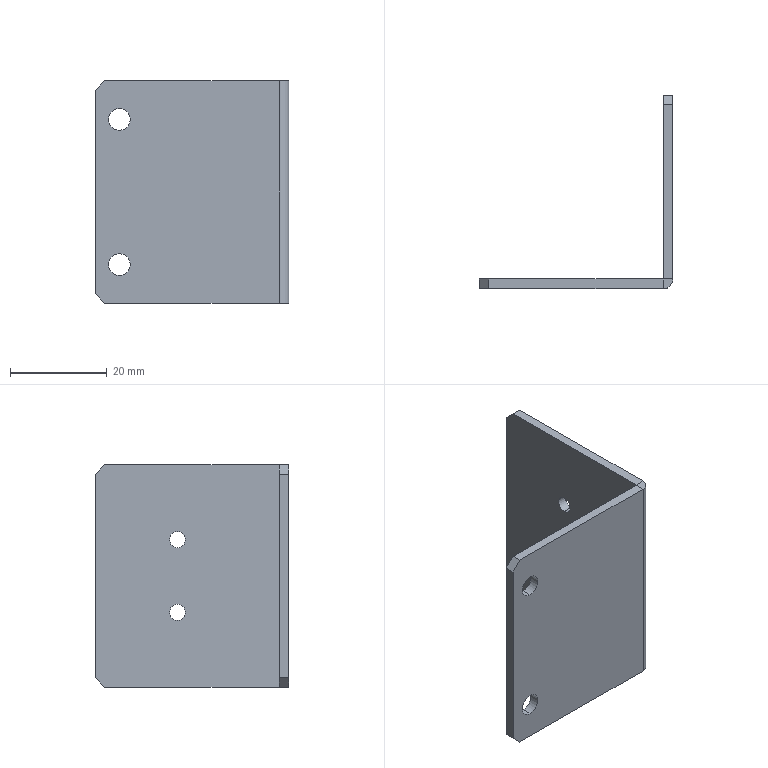Part | NX | features BREP 1 | 1 solid | 26 faces | box 40 x 40 x 46 mm | volume 7022 mm3 | plane 16 | cylinder 10 | commonest cylinder face diameters 3.3 x4 4.5 x4 0.02 x1 4.02 x1
STEP:
#1=CARTESIAN_POINT('',(0.,23.,5.85));
#2=VERTEX_POINT('',#1);
#3=CARTESIAN_POINT('',(0.,23.,9.15));
#4=VERTEX_POINT('',#3);
#5=CARTESIAN_POINT('',(0.,23.,7.5));
#6=DIRECTION('',(-1.,0.,0.));
#7=DIRECTION('',(0.,0.,1.));
#8=AXIS2_PLACEMENT_3D('',#5,#6,#7);
#9=CIRCLE('',#8,1.65);
#10=EDGE_CURVE('',#2,#4,#9,.T.);
#11=ORIENTED_EDGE('',*,*,#10,.F.);
#12=CARTESIAN_POINT('',(-2.,23.,5.85));
#13=VERTEX_POINT('',#12);
#14=CARTESIAN_POINT('',(-2.,23.,5.85));
#15=DIRECTION('',(-1.,0.,0.));
#16=VECTOR('',#15,1000.);
#17=LINE('',#14,#16);
#18=EDGE_CURVE('',#13,#2,#17,.F.);
#19=ORIENTED_EDGE('',*,*,#18,.F.);
#20=CARTESIAN_POINT('',(-2.,23.,9.15));
#21=VERTEX_POINT('',#20);
#22=CARTESIAN_POINT('',(-2.,23.,7.5));
#23=DIRECTION('',(-1.,0.,0.));
#24=DIRECTION('',(0.,0.,1.));
#25=AXIS2_PLACEMENT_3D('',#22,#23,#24);
#26=CIRCLE('',#25,1.65);
#27=EDGE_CURVE('',#13,#21,#26,.T.);
#28=ORIENTED_EDGE('',*,*,#27,.T.);
#29=CARTESIAN_POINT('',(-2.,23.,9.15));
#30=DIRECTION('',(-1.,0.,0.));
#31=VECTOR('',#30,1000.);
#32=LINE('',#29,#31);
#33=EDGE_CURVE('',#21,#4,#32,.F.);
#34=ORIENTED_EDGE('',*,*,#33,.T.);
#35=EDGE_LOOP('',(#11,#19,#28,#34));
#36=FACE_BOUND('',#35,.T.);
#37=CARTESIAN_POINT('',(-2.,23.,7.5));
#38=DIRECTION('',(-1.,0.,0.));
#39=DIRECTION('',(0.,0.,1.));
#40=AXIS2_PLACEMENT_3D('',#37,#38,#39);
#41=CYLINDRICAL_SURFACE('',#40,1.65);
#42=ADVANCED_FACE('',(#36),#41,.F.);
#43=CARTESIAN_POINT('',(0.,23.,-9.15));
#44=VERTEX_POINT('',#43);
#45=CARTESIAN_POINT('',(0.,23.,-5.85));
#46=VERTEX_POINT('',#45);
#47=CARTESIAN_POINT('',(0.,23.,-7.5));
#48=DIRECTION('',(-1.,0.,0.));
#49=DIRECTION('',(0.,0.,1.));
#50=AXIS2_PLACEMENT_3D('',#47,#48,#49);
#51=CIRCLE('',#50,1.65);
#52=EDGE_CURVE('',#44,#46,#51,.T.);
#53=ORIENTED_EDGE('',*,*,#52,.F.);
#54=CARTESIAN_POINT('',(-2.,23.,-9.15));
#55=VERTEX_POINT('',#54);
#56=CARTESIAN_POINT('',(-2.,23.,-9.15));
#57=DIRECTION('',(-1.,0.,0.));
#58=VECTOR('',#57,1000.);
#59=LINE('',#56,#58);
#60=EDGE_CURVE('',#55,#44,#59,.F.);
#61=ORIENTED_EDGE('',*,*,#60,.F.);
#62=CARTESIAN_POINT('',(-2.,23.,-5.85));
#63=VERTEX_POINT('',#62);
#64=CARTESIAN_POINT('',(-2.,23.,-7.5));
#65=DIRECTION('',(-1.,0.,0.));
#66=DIRECTION('',(0.,0.,1.));
#67=AXIS2_PLACEMENT_3D('',#64,#65,#66);
#68=CIRCLE('',#67,1.65);
#69=EDGE_CURVE('',#55,#63,#68,.T.);
#70=ORIENTED_EDGE('',*,*,#69,.T.);
#71=CARTESIAN_POINT('',(-2.,23.,-5.85));
#72=DIRECTION('',(-1.,0.,0.));
#73=VECTOR('',#72,1000.);
#74=LINE('',#71,#73);
#75=EDGE_CURVE('',#63,#46,#74,.F.);
#76=ORIENTED_EDGE('',*,*,#75,.T.);
#77=EDGE_LOOP('',(#53,#61,#70,#76));
#78=FACE_BOUND('',#77,.T.);
#79=CARTESIAN_POINT('',(-2.,23.,-7.5));
#80=DIRECTION('',(-1.,0.,0.));
#81=DIRECTION('',(0.,0.,1.));
#82=AXIS2_PLACEMENT_3D('',#79,#80,#81);
#83=CYLINDRICAL_SURFACE('',#82,1.65);
#84=ADVANCED_FACE('',(#78),#83,.F.);
#85=CARTESIAN_POINT('',(-35.,0.,-12.75));
#86=VERTEX_POINT('',#85);
#87=CARTESIAN_POINT('',(-35.,0.,-17.25));
#88=VERTEX_POINT('',#87);
#89=CARTESIAN_POINT('',(-35.,0.,-15.));
#90=DIRECTION('',(0.,-1.,0.));
#91=DIRECTION('',(1.,0.,0.));
#92=AXIS2_PLACEMENT_3D('',#89,#90,#91);
#93=CIRCLE('',#92,2.25);
#94=EDGE_CURVE('',#86,#88,#93,.T.);
#95=ORIENTED_EDGE('',*,*,#94,.T.);
#96=CARTESIAN_POINT('',(-35.,2.,-17.25));
#97=VERTEX_POINT('',#96);
#98=CARTESIAN_POINT('',(-35.,2.,-17.25));
#99=DIRECTION('',(0.,1.,0.));
#100=VECTOR('',#99,1000.);
#101=LINE('',#98,#100);
#102=EDGE_CURVE('',#97,#88,#101,.F.);
#103=ORIENTED_EDGE('',*,*,#102,.F.);
#104=CARTESIAN_POINT('',(-35.,2.,-12.75));
#105=VERTEX_POINT('',#104);
#106=CARTESIAN_POINT('',(-35.,2.,-15.));
#107=DIRECTION('',(0.,1.,0.));
#108=DIRECTION('',(0.,0.,1.));
#109=AXIS2_PLACEMENT_3D('',#106,#107,#108);
#110=CIRCLE('',#109,2.25);
#111=EDGE_CURVE('',#97,#105,#110,.T.);
#112=ORIENTED_EDGE('',*,*,#111,.T.);
#113=CARTESIAN_POINT('',(-35.,2.,-12.75));
#114=DIRECTION('',(0.,1.,0.));
#115=VECTOR('',#114,1000.);
#116=LINE('',#113,#115);
#117=EDGE_CURVE('',#105,#86,#116,.F.);
#118=ORIENTED_EDGE('',*,*,#117,.T.);
#119=EDGE_LOOP('',(#95,#103,#112,#118));
#120=FACE_BOUND('',#119,.T.);
#121=CARTESIAN_POINT('',(-35.,2.,-15.));
#122=DIRECTION('',(0.,1.,0.));
#123=DIRECTION('',(0.,0.,1.));
#124=AXIS2_PLACEMENT_3D('',#121,#122,#123);
#125=CYLINDRICAL_SURFACE('',#124,2.25);
#126=ADVANCED_FACE('',(#120),#125,.F.);
#127=CARTESIAN_POINT('',(-35.,0.,17.25));
#128=VERTEX_POINT('',#127);
#129=CARTESIAN_POINT('',(-35.,0.,12.75));
#130=VERTEX_POINT('',#129);
#131=CARTESIAN_POINT('',(-35.,0.,15.));
#132=DIRECTION('',(0.,-1.,0.));
#133=DIRECTION('',(1.,0.,0.));
#134=AXIS2_PLACEMENT_3D('',#131,#132,#133);
#135=CIRCLE('',#134,2.25);
#136=EDGE_CURVE('',#128,#130,#135,.T.);
#137=ORIENTED_EDGE('',*,*,#136,.T.);
#138=CARTESIAN_POINT('',(-35.,2.,12.75));
#139=VERTEX_POINT('',#138);
#140=CARTESIAN_POINT('',(-35.,2.,12.75));
#141=DIRECTION('',(0.,1.,0.));
#142=VECTOR('',#141,1000.);
#143=LINE('',#140,#142);
#144=EDGE_CURVE('',#139,#130,#143,.F.);
#145=ORIENTED_EDGE('',*,*,#144,.F.);
#146=CARTESIAN_POINT('',(-35.,2.,17.25));
#147=VERTEX_POINT('',#146);
#148=CARTESIAN_POINT('',(-35.,2.,15.));
#149=DIRECTION('',(0.,1.,0.));
#150=DIRECTION('',(0.,0.,1.));
#151=AXIS2_PLACEMENT_3D('',#148,#149,#150);
#152=CIRCLE('',#151,2.25);
#153=EDGE_CURVE('',#139,#147,#152,.T.);
#154=ORIENTED_EDGE('',*,*,#153,.T.);
#155=CARTESIAN_POINT('',(-35.,2.,17.25));
#156=DIRECTION('',(0.,1.,0.));
#157=VECTOR('',#156,1000.);
#158=LINE('',#155,#157);
#159=EDGE_CURVE('',#147,#128,#158,.F.);
#160=ORIENTED_EDGE('',*,*,#159,.T.);
#161=EDGE_LOOP('',(#137,#145,#154,#160));
#162=FACE_BOUND('',#161,.T.);
#163=CARTESIAN_POINT('',(-35.,2.,15.));
#164=DIRECTION('',(0.,1.,0.));
#165=DIRECTION('',(0.,0.,1.));
#166=AXIS2_PLACEMENT_3D('',#163,#164,#165);
#167=CYLINDRICAL_SURFACE('',#166,2.25);
#168=ADVANCED_FACE('',(#162),#167,.F.);
#169=CARTESIAN_POINT('',(-2.01,0.,23.));
#170=VERTEX_POINT('',#169);
#171=CARTESIAN_POINT('',(-2.01,2.,23.));
#172=VERTEX_POINT('',#171);
#173=CARTESIAN_POINT('',(-2.01,0.,23.));
#174=DIRECTION('',(0.,1.,0.));
#175=VECTOR('',#174,1000.);
#176=LINE('',#173,#175);
#177=EDGE_CURVE('',#170,#172,#176,.T.);
#178=ORIENTED_EDGE('',*,*,#177,.F.);
#179=CARTESIAN_POINT('',(0.,2.01,23.));
#180=VERTEX_POINT('',#179);
#181=CARTESIAN_POINT('',(-2.01,2.01,23.));
#182=DIRECTION('',(0.,0.,-1.));
#183=DIRECTION('',(1.,0.,0.));
#184=AXIS2_PLACEMENT_3D('',#181,#182,#183);
#185=CIRCLE('',#184,2.01);
#186=EDGE_CURVE('',#180,#170,#185,.T.);
#187=ORIENTED_EDGE('',*,*,#186,.F.);
#188=CARTESIAN_POINT('',(-2.,2.01,23.));
#189=VERTEX_POINT('',#188);
#190=CARTESIAN_POINT('',(-2.,2.01,23.));
#191=DIRECTION('',(1.,0.,0.));
#192=VECTOR('',#191,1000.);
#193=LINE('',#190,#192);
#194=EDGE_CURVE('',#189,#180,#193,.T.);
#195=ORIENTED_EDGE('',*,*,#194,.F.);
#196=CARTESIAN_POINT('',(-2.01,2.01,23.));
#197=DIRECTION('',(0.,0.,-1.));
#198=DIRECTION('',(1.,0.,0.));
#199=AXIS2_PLACEMENT_3D('',#196,#197,#198);
#200=CIRCLE('',#199,0.01);
#201=EDGE_CURVE('',#189,#172,#200,.T.);
#202=ORIENTED_EDGE('',*,*,#201,.T.);
#203=EDGE_LOOP('',(#178,#187,#195,#202));
#204=FACE_BOUND('',#203,.T.);
#205=CARTESIAN_POINT('',(-2.01,0.,23.));
#206=DIRECTION('',(0.,0.,1.));
#207=DIRECTION('',(1.,0.,0.));
#208=AXIS2_PLACEMENT_3D('',#205,#206,#207);
#209=PLANE('',#208);
#210=ADVANCED_FACE('',(#204),#209,.T.);
#211=CARTESIAN_POINT('',(-38.,2.,23.));
#212=VERTEX_POINT('',#211);
#213=CARTESIAN_POINT('',(0.,2.,23.));
#214=DIRECTION('',(-1.,0.,0.));
#215=VECTOR('',#214,1000.);
#216=LINE('',#213,#215);
#217=EDGE_CURVE('',#172,#212,#216,.T.);
#218=ORIENTED_EDGE('',*,*,#217,.T.);
#219=CARTESIAN_POINT('',(-38.,0.,23.));
#220=VERTEX_POINT('',#219);
#221=CARTESIAN_POINT('',(-38.,2.01,23.));
#222=DIRECTION('',(0.,-1.,0.));
#223=VECTOR('',#222,1000.);
#224=LINE('',#221,#223);
#225=EDGE_CURVE('',#212,#220,#224,.T.);
#226=ORIENTED_EDGE('',*,*,#225,.T.);
#227=CARTESIAN_POINT('',(0.,0.,23.));
#228=DIRECTION('',(-1.,0.,0.));
#229=VECTOR('',#228,1000.);
#230=LINE('',#227,#229);
#231=EDGE_CURVE('',#170,#220,#230,.T.);
#232=ORIENTED_EDGE('',*,*,#231,.F.);
#233=ORIENTED_EDGE('',*,*,#177,.T.);
#234=EDGE_LOOP('',(#218,#226,#232,#233));
#235=FACE_BOUND('',#234,.T.);
#236=CARTESIAN_POINT('',(-2.,2.01,23.));
#237=DIRECTION('',(0.,0.,1.));
#238=DIRECTION('',(1.,0.,0.));
#239=AXIS2_PLACEMENT_3D('',#236,#237,#238);
#240=PLANE('',#239);
#241=ADVANCED_FACE('',(#235),#240,.T.);
#242=CARTESIAN_POINT('',(0.,2.01,-23.));
#243=VERTEX_POINT('',#242);
#244=CARTESIAN_POINT('',(-2.,2.01,-23.));
#245=VERTEX_POINT('',#244);
#246=CARTESIAN_POINT('',(0.,2.01,-23.));
#247=DIRECTION('',(-1.,0.,0.));
#248=VECTOR('',#247,1000.);
#249=LINE('',#246,#248);
#250=EDGE_CURVE('',#243,#245,#249,.T.);
#251=ORIENTED_EDGE('',*,*,#250,.F.);
#252=CARTESIAN_POINT('',(-2.01,0.,-23.));
#253=VERTEX_POINT('',#252);
#254=CARTESIAN_POINT('',(-2.01,2.01,-23.));
#255=DIRECTION('',(0.,0.,-1.));
#256=DIRECTION('',(1.,0.,0.));
#257=AXIS2_PLACEMENT_3D('',#254,#255,#256);
#258=CIRCLE('',#257,2.01);
#259=EDGE_CURVE('',#243,#253,#258,.T.);
#260=ORIENTED_EDGE('',*,*,#259,.T.);
#261=CARTESIAN_POINT('',(-2.01,2.,-23.));
#262=VERTEX_POINT('',#261);
#263=CARTESIAN_POINT('',(-2.01,2.,-23.));
#264=DIRECTION('',(0.,-1.,0.));
#265=VECTOR('',#264,1000.);
#266=LINE('',#263,#265);
#267=EDGE_CURVE('',#262,#253,#266,.T.);
#268=ORIENTED_EDGE('',*,*,#267,.F.);
#269=CARTESIAN_POINT('',(-2.01,2.01,-23.));
#270=DIRECTION('',(0.,0.,-1.));
#271=DIRECTION('',(1.,0.,0.));
#272=AXIS2_PLACEMENT_3D('',#269,#270,#271);
#273=CIRCLE('',#272,0.01);
#274=EDGE_CURVE('',#245,#262,#273,.T.);
#275=ORIENTED_EDGE('',*,*,#274,.F.);
#276=EDGE_LOOP('',(#251,#260,#268,#275));
#277=FACE_BOUND('',#276,.T.);
#278=CARTESIAN_POINT('',(0.,2.01,-23.));
#279=DIRECTION('',(0.,0.,-1.));
#280=DIRECTION('',(0.,-1.,0.));
#281=AXIS2_PLACEMENT_3D('',#278,#279,#280);
#282=PLANE('',#281);
#283=ADVANCED_FACE('',(#277),#282,.T.);
#284=CARTESIAN_POINT('',(-2.,38.,-23.));
#285=VERTEX_POINT('',#284);
#286=CARTESIAN_POINT('',(-2.,40.,-23.));
#287=DIRECTION('',(0.,-1.,0.));
#288=VECTOR('',#287,1000.);
#289=LINE('',#286,#288);
#290=EDGE_CURVE('',#285,#245,#289,.T.);
#291=ORIENTED_EDGE('',*,*,#290,.F.);
#292=CARTESIAN_POINT('',(0.,38.,-23.));
#293=VERTEX_POINT('',#292);
#294=CARTESIAN_POINT('',(-2.01,38.,-23.));
#295=DIRECTION('',(1.,0.,0.));
#296=VECTOR('',#295,1000.);
#297=LINE('',#294,#296);
#298=EDGE_CURVE('',#285,#293,#297,.T.);
#299=ORIENTED_EDGE('',*,*,#298,.T.);
#300=CARTESIAN_POINT('',(0.,40.,-23.));
#301=DIRECTION('',(0.,-1.,0.));
#302=VECTOR('',#301,1000.);
#303=LINE('',#300,#302);
#304=EDGE_CURVE('',#293,#243,#303,.T.);
#305=ORIENTED_EDGE('',*,*,#304,.T.);
#306=ORIENTED_EDGE('',*,*,#250,.T.);
#307=EDGE_LOOP('',(#291,#299,#305,#306));
#308=FACE_BOUND('',#307,.T.);
#309=CARTESIAN_POINT('',(-2.01,2.,-23.));
#310=DIRECTION('',(0.,0.,-1.));
#311=DIRECTION('',(0.,-1.,0.));
#312=AXIS2_PLACEMENT_3D('',#309,#310,#311);
#313=PLANE('',#312);
#314=ADVANCED_FACE('',(#308),#313,.T.);
#315=CARTESIAN_POINT('',(-40.,2.,21.));
#316=VERTEX_POINT('',#315);
#317=CARTESIAN_POINT('',(-40.,2.,-21.));
#318=VERTEX_POINT('',#317);
#319=CARTESIAN_POINT('',(-40.,2.,23.));
#320=DIRECTION('',(0.,0.,-1.));
#321=VECTOR('',#320,1000.);
#322=LINE('',#319,#321);
#323=EDGE_CURVE('',#316,#318,#322,.T.);
#324=ORIENTED_EDGE('',*,*,#323,.F.);
#325=CARTESIAN_POINT('',(-40.,2.,21.));
#326=DIRECTION('',(0.7071,0.,0.7071));
#327=VECTOR('',#326,1000.);
#328=LINE('',#325,#327);
#329=EDGE_CURVE('',#316,#212,#328,.T.);
#330=ORIENTED_EDGE('',*,*,#329,.T.);
#331=ORIENTED_EDGE('',*,*,#217,.F.);
#332=CARTESIAN_POINT('',(-2.01,2.,23.));
#333=DIRECTION('',(0.,0.,-1.));
#334=VECTOR('',#333,1000.);
#335=LINE('',#332,#334);
#336=EDGE_CURVE('',#172,#262,#335,.T.);
#337=ORIENTED_EDGE('',*,*,#336,.T.);
#338=CARTESIAN_POINT('',(-38.,2.,-23.));
#339=VERTEX_POINT('',#338);
#340=CARTESIAN_POINT('',(0.,2.,-23.));
#341=DIRECTION('',(-1.,0.,0.));
#342=VECTOR('',#341,1000.);
#343=LINE('',#340,#342);
#344=EDGE_CURVE('',#262,#339,#343,.T.);
#345=ORIENTED_EDGE('',*,*,#344,.T.);
#346=CARTESIAN_POINT('',(-38.,2.,-23.));
#347=DIRECTION('',(-0.7071,0.,0.7071));
#348=VECTOR('',#347,1000.);
#349=LINE('',#346,#348);
#350=EDGE_CURVE('',#339,#318,#349,.T.);
#351=ORIENTED_EDGE('',*,*,#350,.T.);
#352=EDGE_LOOP('',(#324,#330,#331,#337,#345,#351));
#353=FACE_BOUND('',#352,.T.);
#354=CARTESIAN_POINT('',(-35.,2.,-15.));
#355=DIRECTION('',(0.,1.,0.));
#356=DIRECTION('',(0.,0.,1.));
#357=AXIS2_PLACEMENT_3D('',#354,#355,#356);
#358=CIRCLE('',#357,2.25);
#359=EDGE_CURVE('',#105,#97,#358,.T.);
#360=ORIENTED_EDGE('',*,*,#359,.F.);
#361=ORIENTED_EDGE('',*,*,#111,.F.);
#362=EDGE_LOOP('',(#360,#361));
#363=FACE_BOUND('',#362,.T.);
#364=CARTESIAN_POINT('',(-35.,2.,15.));
#365=DIRECTION('',(0.,1.,0.));
#366=DIRECTION('',(0.,0.,1.));
#367=AXIS2_PLACEMENT_3D('',#364,#365,#366);
#368=CIRCLE('',#367,2.25);
#369=EDGE_CURVE('',#147,#139,#368,.T.);
#370=ORIENTED_EDGE('',*,*,#369,.F.);
#371=ORIENTED_EDGE('',*,*,#153,.F.);
#372=EDGE_LOOP('',(#370,#371));
#373=FACE_BOUND('',#372,.T.);
#374=CARTESIAN_POINT('',(0.,2.,23.));
#375=DIRECTION('',(0.,-1.,0.));
#376=DIRECTION('',(0.,0.,-1.));
#377=AXIS2_PLACEMENT_3D('',#374,#375,#376);
#378=PLANE('',#377);
#379=ADVANCED_FACE('',(#353,#363,#373),#378,.F.);
#380=CARTESIAN_POINT('',(-40.,0.,21.));
#381=VERTEX_POINT('',#380);
#382=CARTESIAN_POINT('',(-40.,0.,-21.));
#383=VERTEX_POINT('',#382);
#384=CARTESIAN_POINT('',(-40.,0.,23.));
#385=DIRECTION('',(0.,0.,-1.));
#386=VECTOR('',#385,1000.);
#387=LINE('',#384,#386);
#388=EDGE_CURVE('',#381,#383,#387,.T.);
#389=ORIENTED_EDGE('',*,*,#388,.F.);
#390=CARTESIAN_POINT('',(-40.,0.,21.));
#391=DIRECTION('',(0.,1.,0.));
#392=VECTOR('',#391,1000.);
#393=LINE('',#390,#392);
#394=EDGE_CURVE('',#381,#316,#393,.T.);
#395=ORIENTED_EDGE('',*,*,#394,.T.);
#396=ORIENTED_EDGE('',*,*,#323,.T.);
#397=CARTESIAN_POINT('',(-40.,0.,-21.));
#398=DIRECTION('',(0.,-1.,0.));
#399=VECTOR('',#398,1000.);
#400=LINE('',#397,#399);
#401=EDGE_CURVE('',#318,#383,#400,.T.);
#402=ORIENTED_EDGE('',*,*,#401,.T.);
#403=EDGE_LOOP('',(#389,#395,#396,#402));
#404=FACE_BOUND('',#403,.T.);
#405=CARTESIAN_POINT('',(-40.,0.,23.));
#406=DIRECTION('',(-1.,0.,0.));
#407=DIRECTION('',(0.,0.,1.));
#408=AXIS2_PLACEMENT_3D('',#405,#406,#407);
#409=PLANE('',#408);
#410=ADVANCED_FACE('',(#404),#409,.T.);
#411=ORIENTED_EDGE('',*,*,#231,.T.);
#412=CARTESIAN_POINT('',(-19.,0.,42.));
#413=DIRECTION('',(-0.7071,0.,-0.7071));
#414=VECTOR('',#413,1000.);
#415=LINE('',#412,#414);
#416=EDGE_CURVE('',#220,#381,#415,.T.);
#417=ORIENTED_EDGE('',*,*,#416,.T.);
#418=ORIENTED_EDGE('',*,*,#388,.T.);
#419=CARTESIAN_POINT('',(-38.,0.,-23.));
#420=VERTEX_POINT('',#419);
#421=CARTESIAN_POINT('',(-42.,0.,-19.));
#422=DIRECTION('',(0.7071,0.,-0.7071));
#423=VECTOR('',#422,1000.);
#424=LINE('',#421,#423);
#425=EDGE_CURVE('',#383,#420,#424,.T.);
#426=ORIENTED_EDGE('',*,*,#425,.T.);
#427=CARTESIAN_POINT('',(0.,0.,-23.));
#428=DIRECTION('',(-1.,0.,0.));
#429=VECTOR('',#428,1000.);
#430=LINE('',#427,#429);
#431=EDGE_CURVE('',#253,#420,#430,.T.);
#432=ORIENTED_EDGE('',*,*,#431,.F.);
#433=CARTESIAN_POINT('',(-2.01,0.,23.));
#434=DIRECTION('',(0.,0.,-1.));
#435=VECTOR('',#434,1000.);
#436=LINE('',#433,#435);
#437=EDGE_CURVE('',#170,#253,#436,.T.);
#438=ORIENTED_EDGE('',*,*,#437,.F.);
#439=EDGE_LOOP('',(#411,#417,#418,#426,#432,#438));
#440=FACE_BOUND('',#439,.T.);
#441=ORIENTED_EDGE('',*,*,#94,.F.);
#442=CARTESIAN_POINT('',(-35.,0.,-15.));
#443=DIRECTION('',(0.,-1.,0.));
#444=DIRECTION('',(1.,0.,0.));
#445=AXIS2_PLACEMENT_3D('',#442,#443,#444);
#446=CIRCLE('',#445,2.25);
#447=EDGE_CURVE('',#88,#86,#446,.T.);
#448=ORIENTED_EDGE('',*,*,#447,.F.);
#449=EDGE_LOOP('',(#441,#448));
#450=FACE_BOUND('',#449,.T.);
#451=ORIENTED_EDGE('',*,*,#136,.F.);
#452=CARTESIAN_POINT('',(-35.,0.,15.));
#453=DIRECTION('',(0.,-1.,0.));
#454=DIRECTION('',(1.,0.,0.));
#455=AXIS2_PLACEMENT_3D('',#452,#453,#454);
#456=CIRCLE('',#455,2.25);
#457=EDGE_CURVE('',#130,#128,#456,.T.);
#458=ORIENTED_EDGE('',*,*,#457,.F.);
#459=EDGE_LOOP('',(#451,#458));
#460=FACE_BOUND('',#459,.T.);
#461=CARTESIAN_POINT('',(0.,0.,23.));
#462=DIRECTION('',(0.,-1.,0.));
#463=DIRECTION('',(0.,0.,-1.));
#464=AXIS2_PLACEMENT_3D('',#461,#462,#463);
#465=PLANE('',#464);
#466=ADVANCED_FACE('',(#440,#450,#460),#465,.T.);
#467=ORIENTED_EDGE('',*,*,#259,.F.);
#468=CARTESIAN_POINT('',(0.,2.01,23.));
#469=DIRECTION('',(0.,0.,-1.));
#470=VECTOR('',#469,1000.);
#471=LINE('',#468,#470);
#472=EDGE_CURVE('',#180,#243,#471,.T.);
#473=ORIENTED_EDGE('',*,*,#472,.F.);
#474=ORIENTED_EDGE('',*,*,#186,.T.);
#475=ORIENTED_EDGE('',*,*,#437,.T.);
#476=EDGE_LOOP('',(#467,#473,#474,#475));
#477=FACE_BOUND('',#476,.T.);
#478=CARTESIAN_POINT('',(-2.01,2.01,23.));
#479=DIRECTION('',(0.,0.,-1.));
#480=DIRECTION('',(-1.,0.,0.));
#481=AXIS2_PLACEMENT_3D('',#478,#479,#480);
#482=CYLINDRICAL_SURFACE('',#481,2.01);
#483=ADVANCED_FACE('',(#477),#482,.T.);
#484=ORIENTED_EDGE('',*,*,#304,.F.);
#485=CARTESIAN_POINT('',(0.,40.,-21.));
#486=VERTEX_POINT('',#485);
#487=CARTESIAN_POINT('',(0.,62.,1.));
#488=DIRECTION('',(0.,0.7071,0.7071));
#489=VECTOR('',#488,1000.);
#490=LINE('',#487,#489);
#491=EDGE_CURVE('',#293,#486,#490,.T.);
#492=ORIENTED_EDGE('',*,*,#491,.T.);
#493=CARTESIAN_POINT('',(0.,40.,21.));
#494=VERTEX_POINT('',#493);
#495=CARTESIAN_POINT('',(0.,40.,23.));
#496=DIRECTION('',(0.,0.,-1.));
#497=VECTOR('',#496,1000.);
#498=LINE('',#495,#497);
#499=EDGE_CURVE('',#494,#486,#498,.T.);
#500=ORIENTED_EDGE('',*,*,#499,.F.);
#501=CARTESIAN_POINT('',(0.,38.,23.));
#502=VERTEX_POINT('',#501);
#503=CARTESIAN_POINT('',(0.,39.,22.));
#504=DIRECTION('',(0.,-0.7071,0.7071));
#505=VECTOR('',#504,1000.);
#506=LINE('',#503,#505);
#507=EDGE_CURVE('',#494,#502,#506,.T.);
#508=ORIENTED_EDGE('',*,*,#507,.T.);
#509=CARTESIAN_POINT('',(0.,40.,23.));
#510=DIRECTION('',(0.,-1.,0.));
#511=VECTOR('',#510,1000.);
#512=LINE('',#509,#511);
#513=EDGE_CURVE('',#502,#180,#512,.T.);
#514=ORIENTED_EDGE('',*,*,#513,.T.);
#515=ORIENTED_EDGE('',*,*,#472,.T.);
#516=EDGE_LOOP('',(#484,#492,#500,#508,#514,#515));
#517=FACE_BOUND('',#516,.T.);
#518=CARTESIAN_POINT('',(0.,23.,7.5));
#519=DIRECTION('',(-1.,0.,0.));
#520=DIRECTION('',(0.,0.,1.));
#521=AXIS2_PLACEMENT_3D('',#518,#519,#520);
#522=CIRCLE('',#521,1.65);
#523=EDGE_CURVE('',#4,#2,#522,.T.);
#524=ORIENTED_EDGE('',*,*,#523,.T.);
#525=ORIENTED_EDGE('',*,*,#10,.T.);
#526=EDGE_LOOP('',(#524,#525));
#527=FACE_BOUND('',#526,.T.);
#528=CARTESIAN_POINT('',(0.,23.,-7.5));
#529=DIRECTION('',(-1.,0.,0.));
#530=DIRECTION('',(0.,0.,1.));
#531=AXIS2_PLACEMENT_3D('',#528,#529,#530);
#532=CIRCLE('',#531,1.65);
#533=EDGE_CURVE('',#46,#44,#532,.T.);
#534=ORIENTED_EDGE('',*,*,#533,.T.);
#535=ORIENTED_EDGE('',*,*,#52,.T.);
#536=EDGE_LOOP('',(#534,#535));
#537=FACE_BOUND('',#536,.T.);
#538=CARTESIAN_POINT('',(0.,40.,23.));
#539=DIRECTION('',(1.,0.,0.));
#540=DIRECTION('',(0.,-1.,0.));
#541=AXIS2_PLACEMENT_3D('',#538,#539,#540);
#542=PLANE('',#541);
#543=ADVANCED_FACE('',(#517,#527,#537),#542,.T.);
#544=ORIENTED_EDGE('',*,*,#499,.T.);
#545=CARTESIAN_POINT('',(-2.,40.,-21.));
#546=VERTEX_POINT('',#545);
#547=CARTESIAN_POINT('',(-2.,40.,-21.));
#548=DIRECTION('',(-1.,0.,0.));
#549=VECTOR('',#548,1000.);
#550=LINE('',#547,#549);
#551=EDGE_CURVE('',#486,#546,#550,.T.);
#552=ORIENTED_EDGE('',*,*,#551,.T.);
#553=CARTESIAN_POINT('',(-2.,40.,21.));
#554=VERTEX_POINT('',#553);
#555=CARTESIAN_POINT('',(-2.,40.,23.));
#556=DIRECTION('',(0.,0.,-1.));
#557=VECTOR('',#556,1000.);
#558=LINE('',#555,#557);
#559=EDGE_CURVE('',#554,#546,#558,.T.);
#560=ORIENTED_EDGE('',*,*,#559,.F.);
#561=CARTESIAN_POINT('',(-2.,40.,21.));
#562=DIRECTION('',(1.,0.,0.));
#563=VECTOR('',#562,1000.);
#564=LINE('',#561,#563);
#565=EDGE_CURVE('',#554,#494,#564,.T.);
#566=ORIENTED_EDGE('',*,*,#565,.T.);
#567=EDGE_LOOP('',(#544,#552,#560,#566));
#568=FACE_BOUND('',#567,.T.);
#569=CARTESIAN_POINT('',(-2.,40.,23.));
#570=DIRECTION('',(0.,1.,0.));
#571=DIRECTION('',(1.,0.,0.));
#572=AXIS2_PLACEMENT_3D('',#569,#570,#571);
#573=PLANE('',#572);
#574=ADVANCED_FACE('',(#568),#573,.T.);
#575=ORIENTED_EDGE('',*,*,#559,.T.);
#576=CARTESIAN_POINT('',(-2.,38.,-23.));
#577=DIRECTION('',(0.,-0.7071,-0.7071));
#578=VECTOR('',#577,1000.);
#579=LINE('',#576,#578);
#580=EDGE_CURVE('',#546,#285,#579,.T.);
#581=ORIENTED_EDGE('',*,*,#580,.T.);
#582=ORIENTED_EDGE('',*,*,#290,.T.);
#583=CARTESIAN_POINT('',(-2.,2.01,23.));
#584=DIRECTION('',(0.,0.,-1.));
#585=VECTOR('',#584,1000.);
#586=LINE('',#583,#585);
#587=EDGE_CURVE('',#189,#245,#586,.T.);
#588=ORIENTED_EDGE('',*,*,#587,.F.);
#589=CARTESIAN_POINT('',(-2.,38.,23.));
#590=VERTEX_POINT('',#589);
#591=CARTESIAN_POINT('',(-2.,40.,23.));
#592=DIRECTION('',(0.,-1.,0.));
#593=VECTOR('',#592,1000.);
#594=LINE('',#591,#593);
#595=EDGE_CURVE('',#590,#189,#594,.T.);
#596=ORIENTED_EDGE('',*,*,#595,.F.);
#597=CARTESIAN_POINT('',(-2.,40.,21.));
#598=DIRECTION('',(0.,0.7071,-0.7071));
#599=VECTOR('',#598,1000.);
#600=LINE('',#597,#599);
#601=EDGE_CURVE('',#590,#554,#600,.T.);
#602=ORIENTED_EDGE('',*,*,#601,.T.);
#603=EDGE_LOOP('',(#575,#581,#582,#588,#596,#602));
#604=FACE_BOUND('',#603,.T.);
#605=CARTESIAN_POINT('',(-2.,23.,7.5));
#606=DIRECTION('',(-1.,0.,0.));
#607=DIRECTION('',(0.,0.,1.));
#608=AXIS2_PLACEMENT_3D('',#605,#606,#607);
#609=CIRCLE('',#608,1.65);
#610=EDGE_CURVE('',#21,#13,#609,.T.);
#611=ORIENTED_EDGE('',*,*,#610,.F.);
#612=ORIENTED_EDGE('',*,*,#27,.F.);
#613=EDGE_LOOP('',(#611,#612));
#614=FACE_BOUND('',#613,.T.);
#615=CARTESIAN_POINT('',(-2.,23.,-7.5));
#616=DIRECTION('',(-1.,0.,0.));
#617=DIRECTION('',(0.,0.,1.));
#618=AXIS2_PLACEMENT_3D('',#615,#616,#617);
#619=CIRCLE('',#618,1.65);
#620=EDGE_CURVE('',#63,#55,#619,.T.);
#621=ORIENTED_EDGE('',*,*,#620,.F.);
#622=ORIENTED_EDGE('',*,*,#69,.F.);
#623=EDGE_LOOP('',(#621,#622));
#624=FACE_BOUND('',#623,.T.);
#625=CARTESIAN_POINT('',(-2.,40.,23.));
#626=DIRECTION('',(1.,0.,0.));
#627=DIRECTION('',(0.,-1.,0.));
#628=AXIS2_PLACEMENT_3D('',#625,#626,#627);
#629=PLANE('',#628);
#630=ADVANCED_FACE('',(#604,#614,#624),#629,.F.);
#631=ORIENTED_EDGE('',*,*,#274,.T.);
#632=ORIENTED_EDGE('',*,*,#336,.F.);
#633=ORIENTED_EDGE('',*,*,#201,.F.);
#634=ORIENTED_EDGE('',*,*,#587,.T.);
#635=EDGE_LOOP('',(#631,#632,#633,#634));
#636=FACE_BOUND('',#635,.T.);
#637=CARTESIAN_POINT('',(-2.01,2.01,23.));
#638=DIRECTION('',(0.,0.,-1.));
#639=DIRECTION('',(-1.,0.,0.));
#640=AXIS2_PLACEMENT_3D('',#637,#638,#639);
#641=CYLINDRICAL_SURFACE('',#640,0.01);
#642=ADVANCED_FACE('',(#636),#641,.F.);
#643=ORIENTED_EDGE('',*,*,#513,.F.);
#644=CARTESIAN_POINT('',(-2.01,38.,23.));
#645=DIRECTION('',(-1.,0.,0.));
#646=VECTOR('',#645,1000.);
#647=LINE('',#644,#646);
#648=EDGE_CURVE('',#502,#590,#647,.T.);
#649=ORIENTED_EDGE('',*,*,#648,.T.);
#650=ORIENTED_EDGE('',*,*,#595,.T.);
#651=ORIENTED_EDGE('',*,*,#194,.T.);
#652=EDGE_LOOP('',(#643,#649,#650,#651));
#653=FACE_BOUND('',#652,.T.);
#654=CARTESIAN_POINT('',(-2.01,2.01,23.));
#655=DIRECTION('',(0.,0.,1.));
#656=DIRECTION('',(1.,0.,0.));
#657=AXIS2_PLACEMENT_3D('',#654,#655,#656);
#658=PLANE('',#657);
#659=ADVANCED_FACE('',(#653),#658,.T.);
#660=ORIENTED_EDGE('',*,*,#431,.T.);
#661=CARTESIAN_POINT('',(-38.,2.,-23.));
#662=DIRECTION('',(0.,1.,0.));
#663=VECTOR('',#662,1000.);
#664=LINE('',#661,#663);
#665=EDGE_CURVE('',#420,#339,#664,.T.);
#666=ORIENTED_EDGE('',*,*,#665,.T.);
#667=ORIENTED_EDGE('',*,*,#344,.F.);
#668=ORIENTED_EDGE('',*,*,#267,.T.);
#669=EDGE_LOOP('',(#660,#666,#667,#668));
#670=FACE_BOUND('',#669,.T.);
#671=CARTESIAN_POINT('',(-2.01,2.01,-23.));
#672=DIRECTION('',(0.,0.,1.));
#673=DIRECTION('',(1.,0.,0.));
#674=AXIS2_PLACEMENT_3D('',#671,#672,#673);
#675=PLANE('',#674);
#676=ADVANCED_FACE('',(#670),#675,.F.);
#677=ORIENTED_EDGE('',*,*,#144,.T.);
#678=ORIENTED_EDGE('',*,*,#457,.T.);
#679=ORIENTED_EDGE('',*,*,#159,.F.);
#680=ORIENTED_EDGE('',*,*,#369,.T.);
#681=EDGE_LOOP('',(#677,#678,#679,#680));
#682=FACE_BOUND('',#681,.T.);
#683=CARTESIAN_POINT('',(-35.,2.,15.));
#684=DIRECTION('',(0.,1.,0.));
#685=DIRECTION('',(0.,0.,1.));
#686=AXIS2_PLACEMENT_3D('',#683,#684,#685);
#687=CYLINDRICAL_SURFACE('',#686,2.25);
#688=ADVANCED_FACE('',(#682),#687,.F.);
#689=ORIENTED_EDGE('',*,*,#102,.T.);
#690=ORIENTED_EDGE('',*,*,#447,.T.);
#691=ORIENTED_EDGE('',*,*,#117,.F.);
#692=ORIENTED_EDGE('',*,*,#359,.T.);
#693=EDGE_LOOP('',(#689,#690,#691,#692));
#694=FACE_BOUND('',#693,.T.);
#695=CARTESIAN_POINT('',(-35.,2.,-15.));
#696=DIRECTION('',(0.,1.,0.));
#697=DIRECTION('',(0.,0.,1.));
#698=AXIS2_PLACEMENT_3D('',#695,#696,#697);
#699=CYLINDRICAL_SURFACE('',#698,2.25);
#700=ADVANCED_FACE('',(#694),#699,.F.);
#701=ORIENTED_EDGE('',*,*,#580,.F.);
#702=ORIENTED_EDGE('',*,*,#551,.F.);
#703=ORIENTED_EDGE('',*,*,#491,.F.);
#704=ORIENTED_EDGE('',*,*,#298,.F.);
#705=EDGE_LOOP('',(#701,#702,#703,#704));
#706=FACE_BOUND('',#705,.T.);
#707=CARTESIAN_POINT('',(-2.01,38.,-23.));
#708=DIRECTION('',(0.,-0.7071,0.7071));
#709=DIRECTION('',(-1.,0.,0.));
#710=AXIS2_PLACEMENT_3D('',#707,#708,#709);
#711=PLANE('',#710);
#712=ADVANCED_FACE('',(#706),#711,.F.);
#713=ORIENTED_EDGE('',*,*,#601,.F.);
#714=ORIENTED_EDGE('',*,*,#648,.F.);
#715=ORIENTED_EDGE('',*,*,#507,.F.);
#716=ORIENTED_EDGE('',*,*,#565,.F.);
#717=EDGE_LOOP('',(#713,#714,#715,#716));
#718=FACE_BOUND('',#717,.T.);
#719=CARTESIAN_POINT('',(-2.,40.,21.));
#720=DIRECTION('',(0.,-0.7071,-0.7071));
#721=DIRECTION('',(0.,-0.7071,0.7071));
#722=AXIS2_PLACEMENT_3D('',#719,#720,#721);
#723=PLANE('',#722);
#724=ADVANCED_FACE('',(#718),#723,.F.);
#725=ORIENTED_EDGE('',*,*,#416,.F.);
#726=ORIENTED_EDGE('',*,*,#225,.F.);
#727=ORIENTED_EDGE('',*,*,#329,.F.);
#728=ORIENTED_EDGE('',*,*,#394,.F.);
#729=EDGE_LOOP('',(#725,#726,#727,#728));
#730=FACE_BOUND('',#729,.T.);
#731=CARTESIAN_POINT('',(-40.,0.,21.));
#732=DIRECTION('',(0.7071,0.,-0.7071));
#733=DIRECTION('',(0.,-1.,0.));
#734=AXIS2_PLACEMENT_3D('',#731,#732,#733);
#735=PLANE('',#734);
#736=ADVANCED_FACE('',(#730),#735,.F.);
#737=ORIENTED_EDGE('',*,*,#425,.F.);
#738=ORIENTED_EDGE('',*,*,#401,.F.);
#739=ORIENTED_EDGE('',*,*,#350,.F.);
#740=ORIENTED_EDGE('',*,*,#665,.F.);
#741=EDGE_LOOP('',(#737,#738,#739,#740));
#742=FACE_BOUND('',#741,.T.);
#743=CARTESIAN_POINT('',(-38.,2.01,-23.));
#744=DIRECTION('',(-0.7071,0.,-0.7071));
#745=DIRECTION('',(-0.7071,0.,0.7071));
#746=AXIS2_PLACEMENT_3D('',#743,#744,#745);
#747=PLANE('',#746);
#748=ADVANCED_FACE('',(#742),#747,.T.);
#749=ORIENTED_EDGE('',*,*,#60,.T.);
#750=ORIENTED_EDGE('',*,*,#533,.F.);
#751=ORIENTED_EDGE('',*,*,#75,.F.);
#752=ORIENTED_EDGE('',*,*,#620,.T.);
#753=EDGE_LOOP('',(#749,#750,#751,#752));
#754=FACE_BOUND('',#753,.T.);
#755=CARTESIAN_POINT('',(-2.,23.,-7.5));
#756=DIRECTION('',(-1.,0.,0.));
#757=DIRECTION('',(0.,0.,1.));
#758=AXIS2_PLACEMENT_3D('',#755,#756,#757);
#759=CYLINDRICAL_SURFACE('',#758,1.65);
#760=ADVANCED_FACE('',(#754),#759,.F.);
#761=ORIENTED_EDGE('',*,*,#18,.T.);
#762=ORIENTED_EDGE('',*,*,#523,.F.);
#763=ORIENTED_EDGE('',*,*,#33,.F.);
#764=ORIENTED_EDGE('',*,*,#610,.T.);
#765=EDGE_LOOP('',(#761,#762,#763,#764));
#766=FACE_BOUND('',#765,.T.);
#767=CARTESIAN_POINT('',(-2.,23.,7.5));
#768=DIRECTION('',(-1.,0.,0.));
#769=DIRECTION('',(0.,0.,1.));
#770=AXIS2_PLACEMENT_3D('',#767,#768,#769);
#771=CYLINDRICAL_SURFACE('',#770,1.65);
#772=ADVANCED_FACE('',(#766),#771,.F.);
#773=CLOSED_SHELL('',(#42,#84,#126,#168,#210,#241,#283,#314,#379,#410,#466,#483,#543,#574,#630,#642,#659,#676,#688,#700,#712,#724,#736,#748,#760,#772));
#774=MANIFOLD_SOLID_BREP('',#773);
#775=(LENGTH_UNIT()NAMED_UNIT(*)SI_UNIT(.MILLI.,.METRE.));
#776=UNCERTAINTY_MEASURE_WITH_UNIT(LENGTH_MEASURE(0.00001),#775,'','');
#777=(NAMED_UNIT(*)PLANE_ANGLE_UNIT()SI_UNIT($,.RADIAN.));
#778=(NAMED_UNIT(*)SI_UNIT($,.STERADIAN.)SOLID_ANGLE_UNIT());
#779=(GEOMETRIC_REPRESENTATION_CONTEXT(3)GLOBAL_UNCERTAINTY_ASSIGNED_CONTEXT((#776))GLOBAL_UNIT_ASSIGNED_CONTEXT((#775,#777,#778))REPRESENTATION_CONTEXT('',''));
#780=ADVANCED_BREP_SHAPE_REPRESENTATION('',(#774),#779);